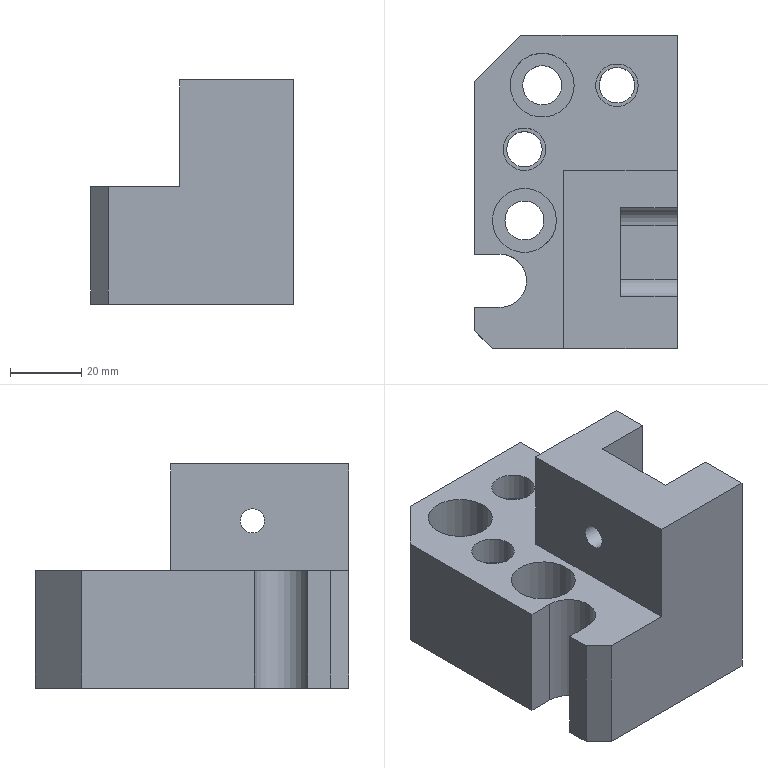Part | STEP file | gslz 2016.10.28-13_id1618_x_t | 1 solid | 36 faces | box 57 x 88 x 63 mm | volume 168012 mm3 | plane 22 | cylinder 13 | cone 1 | commonest cylinder face diameters 10 x4 6.8 x2 11 x2 12 x2 18 x2 15 x1